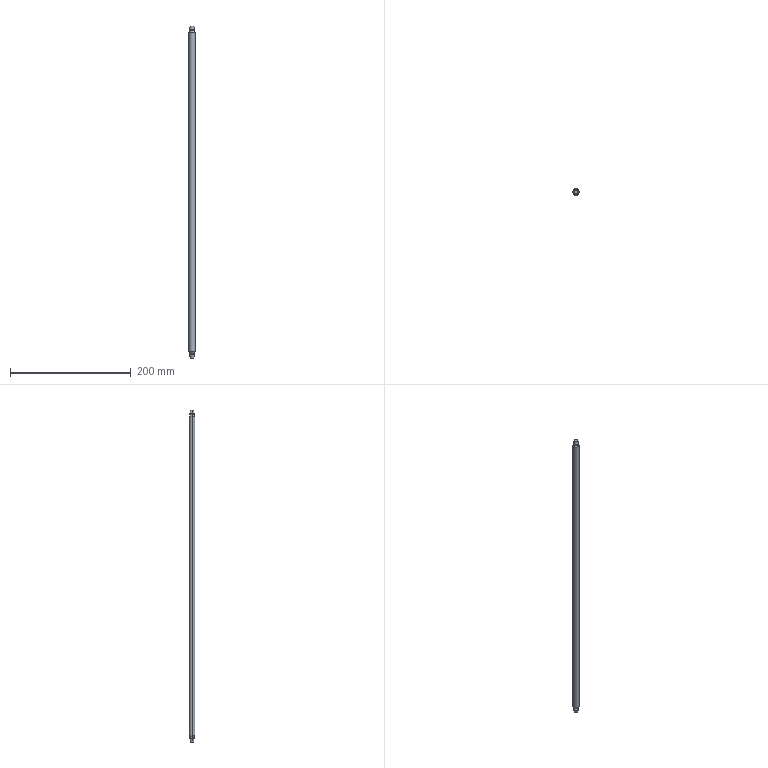Part | SolidWorks | features BaseBody 1 | 1 solid | 16 faces | box 10 x 10 x 550 mm | volume 42463 mm3 | torus 8 | cone 4 | cylinder 2 | plane 2 | commonest cylinder face diameters 10 x2
STEP:
#1=CARTESIAN_POINT('',(-5.,0.,-265.));
#2=VERTEX_POINT('',#1);
#3=CARTESIAN_POINT('',(-3.,0.,-267.));
#4=VERTEX_POINT('',#3);
#5=CARTESIAN_POINT('',(-5.,0.,-267.));
#6=DIRECTION('',(0.,1.,0.));
#7=DIRECTION('',(0.,0.,1.));
#8=AXIS2_PLACEMENT_3D('',#5,#6,#7);
#9=CIRCLE('',#8,2.);
#10=EDGE_CURVE('',#2,#4,#9,.T.);
#11=ORIENTED_EDGE('',*,*,#10,.T.);
#12=CARTESIAN_POINT('',(3.,0.,-267.));
#13=VERTEX_POINT('',#12);
#14=CARTESIAN_POINT('',(0.,0.,-267.));
#15=DIRECTION('',(0.,0.,1.));
#16=DIRECTION('',(1.,0.,0.));
#17=AXIS2_PLACEMENT_3D('',#14,#15,#16);
#18=CIRCLE('',#17,3.);
#19=EDGE_CURVE('',#4,#13,#18,.T.);
#20=ORIENTED_EDGE('',*,*,#19,.T.);
#21=CARTESIAN_POINT('',(5.,0.,-265.));
#22=VERTEX_POINT('',#21);
#23=CARTESIAN_POINT('',(5.,0.,-267.));
#24=DIRECTION('',(0.,-1.,0.));
#25=DIRECTION('',(1.,0.,0.));
#26=AXIS2_PLACEMENT_3D('',#23,#24,#25);
#27=CIRCLE('',#26,2.);
#28=EDGE_CURVE('',#22,#13,#27,.T.);
#29=ORIENTED_EDGE('',*,*,#28,.F.);
#30=CARTESIAN_POINT('',(0.,0.,-265.));
#31=DIRECTION('',(0.,0.,-1.));
#32=DIRECTION('',(-1.,0.,0.));
#33=AXIS2_PLACEMENT_3D('',#30,#31,#32);
#34=CIRCLE('',#33,5.);
#35=EDGE_CURVE('',#22,#2,#34,.T.);
#36=ORIENTED_EDGE('',*,*,#35,.T.);
#37=EDGE_LOOP('',(#11,#20,#29,#36));
#38=FACE_OUTER_BOUND('',#37,.T.);
#39=CARTESIAN_POINT('',(0.,0.,-267.));
#40=DIRECTION('',(0.,0.,1.));
#41=DIRECTION('',(-1.,0.,0.));
#42=AXIS2_PLACEMENT_3D('',#39,#40,#41);
#43=TOROIDAL_SURFACE('',#42,5.,2.);
#44=ADVANCED_FACE('',(#38),#43,.F.);
#45=CARTESIAN_POINT('',(-5.,0.,265.));
#46=VERTEX_POINT('',#45);
#47=CARTESIAN_POINT('',(-3.,0.,267.));
#48=VERTEX_POINT('',#47);
#49=CARTESIAN_POINT('',(-5.,0.,267.));
#50=DIRECTION('',(0.,-1.,0.));
#51=DIRECTION('',(0.,0.,-1.));
#52=AXIS2_PLACEMENT_3D('',#49,#50,#51);
#53=CIRCLE('',#52,2.);
#54=EDGE_CURVE('',#46,#48,#53,.T.);
#55=ORIENTED_EDGE('',*,*,#54,.T.);
#56=CARTESIAN_POINT('',(3.,0.,267.));
#57=VERTEX_POINT('',#56);
#58=CARTESIAN_POINT('',(0.,0.,267.));
#59=DIRECTION('',(0.,0.,-1.));
#60=DIRECTION('',(-1.,0.,0.));
#61=AXIS2_PLACEMENT_3D('',#58,#59,#60);
#62=CIRCLE('',#61,3.);
#63=EDGE_CURVE('',#48,#57,#62,.T.);
#64=ORIENTED_EDGE('',*,*,#63,.T.);
#65=CARTESIAN_POINT('',(5.,0.,265.));
#66=VERTEX_POINT('',#65);
#67=CARTESIAN_POINT('',(5.,0.,267.));
#68=DIRECTION('',(0.,1.,0.));
#69=DIRECTION('',(-1.,0.,0.));
#70=AXIS2_PLACEMENT_3D('',#67,#68,#69);
#71=CIRCLE('',#70,2.);
#72=EDGE_CURVE('',#66,#57,#71,.T.);
#73=ORIENTED_EDGE('',*,*,#72,.F.);
#74=CARTESIAN_POINT('',(0.,0.,265.));
#75=DIRECTION('',(0.,0.,1.));
#76=DIRECTION('',(-1.,0.,0.));
#77=AXIS2_PLACEMENT_3D('',#74,#75,#76);
#78=CIRCLE('',#77,5.);
#79=EDGE_CURVE('',#66,#46,#78,.T.);
#80=ORIENTED_EDGE('',*,*,#79,.T.);
#81=EDGE_LOOP('',(#55,#64,#73,#80));
#82=FACE_OUTER_BOUND('',#81,.T.);
#83=CARTESIAN_POINT('',(0.,0.,267.));
#84=DIRECTION('',(0.,0.,-1.));
#85=DIRECTION('',(-1.,0.,0.));
#86=AXIS2_PLACEMENT_3D('',#83,#84,#85);
#87=TOROIDAL_SURFACE('',#86,5.,2.);
#88=ADVANCED_FACE('',(#82),#87,.F.);
#89=ORIENTED_EDGE('',*,*,#72,.T.);
#90=CARTESIAN_POINT('',(0.,0.,267.));
#91=DIRECTION('',(0.,0.,-1.));
#92=DIRECTION('',(-1.,0.,0.));
#93=AXIS2_PLACEMENT_3D('',#90,#91,#92);
#94=CIRCLE('',#93,3.);
#95=EDGE_CURVE('',#57,#48,#94,.T.);
#96=ORIENTED_EDGE('',*,*,#95,.T.);
#97=ORIENTED_EDGE('',*,*,#54,.F.);
#98=CARTESIAN_POINT('',(0.,0.,265.));
#99=DIRECTION('',(0.,0.,1.));
#100=DIRECTION('',(-1.,0.,0.));
#101=AXIS2_PLACEMENT_3D('',#98,#99,#100);
#102=CIRCLE('',#101,5.);
#103=EDGE_CURVE('',#46,#66,#102,.T.);
#104=ORIENTED_EDGE('',*,*,#103,.T.);
#105=EDGE_LOOP('',(#89,#96,#97,#104));
#106=FACE_OUTER_BOUND('',#105,.T.);
#107=CARTESIAN_POINT('',(0.,0.,267.));
#108=DIRECTION('',(0.,0.,-1.));
#109=DIRECTION('',(-1.,0.,0.));
#110=AXIS2_PLACEMENT_3D('',#107,#108,#109);
#111=TOROIDAL_SURFACE('',#110,5.,2.);
#112=ADVANCED_FACE('',(#106),#111,.F.);
#113=ORIENTED_EDGE('',*,*,#28,.T.);
#114=CARTESIAN_POINT('',(0.,0.,-267.));
#115=DIRECTION('',(0.,0.,1.));
#116=DIRECTION('',(1.,0.,0.));
#117=AXIS2_PLACEMENT_3D('',#114,#115,#116);
#118=CIRCLE('',#117,3.);
#119=EDGE_CURVE('',#13,#4,#118,.T.);
#120=ORIENTED_EDGE('',*,*,#119,.T.);
#121=ORIENTED_EDGE('',*,*,#10,.F.);
#122=CARTESIAN_POINT('',(0.,0.,-265.));
#123=DIRECTION('',(0.,0.,-1.));
#124=DIRECTION('',(-1.,0.,0.));
#125=AXIS2_PLACEMENT_3D('',#122,#123,#124);
#126=CIRCLE('',#125,5.);
#127=EDGE_CURVE('',#2,#22,#126,.T.);
#128=ORIENTED_EDGE('',*,*,#127,.T.);
#129=EDGE_LOOP('',(#113,#120,#121,#128));
#130=FACE_OUTER_BOUND('',#129,.T.);
#131=CARTESIAN_POINT('',(0.,0.,-267.));
#132=DIRECTION('',(0.,0.,1.));
#133=DIRECTION('',(-1.,0.,0.));
#134=AXIS2_PLACEMENT_3D('',#131,#132,#133);
#135=TOROIDAL_SURFACE('',#134,5.,2.);
#136=ADVANCED_FACE('',(#130),#135,.F.);
#137=ORIENTED_EDGE('',*,*,#119,.F.);
#138=CARTESIAN_POINT('',(4.515,0.,-268.94));
#139=VERTEX_POINT('',#138);
#140=CARTESIAN_POINT('',(5.,0.,-267.));
#141=DIRECTION('',(0.,-1.,0.));
#142=DIRECTION('',(1.,0.,0.));
#143=AXIS2_PLACEMENT_3D('',#140,#141,#142);
#144=CIRCLE('',#143,2.);
#145=EDGE_CURVE('',#13,#139,#144,.T.);
#146=ORIENTED_EDGE('',*,*,#145,.T.);
#147=CARTESIAN_POINT('',(-4.515,0.,-268.94));
#148=VERTEX_POINT('',#147);
#149=CARTESIAN_POINT('',(0.,0.,-268.94));
#150=DIRECTION('',(0.,0.,-1.));
#151=DIRECTION('',(1.,0.,0.));
#152=AXIS2_PLACEMENT_3D('',#149,#150,#151);
#153=CIRCLE('',#152,4.515);
#154=EDGE_CURVE('',#148,#139,#153,.T.);
#155=ORIENTED_EDGE('',*,*,#154,.F.);
#156=CARTESIAN_POINT('',(-5.,0.,-267.));
#157=DIRECTION('',(0.,1.,0.));
#158=DIRECTION('',(0.,0.,1.));
#159=AXIS2_PLACEMENT_3D('',#156,#157,#158);
#160=CIRCLE('',#159,2.);
#161=EDGE_CURVE('',#4,#148,#160,.T.);
#162=ORIENTED_EDGE('',*,*,#161,.F.);
#163=EDGE_LOOP('',(#137,#146,#155,#162));
#164=FACE_OUTER_BOUND('',#163,.T.);
#165=CARTESIAN_POINT('',(0.,0.,-267.));
#166=DIRECTION('',(0.,0.,1.));
#167=DIRECTION('',(-1.,0.,0.));
#168=AXIS2_PLACEMENT_3D('',#165,#166,#167);
#169=TOROIDAL_SURFACE('',#168,5.,2.);
#170=ADVANCED_FACE('',(#164),#169,.F.);
#171=ORIENTED_EDGE('',*,*,#95,.F.);
#172=CARTESIAN_POINT('',(4.515,0.,268.94));
#173=VERTEX_POINT('',#172);
#174=CARTESIAN_POINT('',(5.,0.,267.));
#175=DIRECTION('',(0.,1.,0.));
#176=DIRECTION('',(-1.,0.,0.));
#177=AXIS2_PLACEMENT_3D('',#174,#175,#176);
#178=CIRCLE('',#177,2.);
#179=EDGE_CURVE('',#57,#173,#178,.T.);
#180=ORIENTED_EDGE('',*,*,#179,.T.);
#181=CARTESIAN_POINT('',(-4.515,0.,268.94));
#182=VERTEX_POINT('',#181);
#183=CARTESIAN_POINT('',(0.,0.,268.94));
#184=DIRECTION('',(0.,0.,-1.));
#185=DIRECTION('',(1.,0.,0.));
#186=AXIS2_PLACEMENT_3D('',#183,#184,#185);
#187=CIRCLE('',#186,4.515);
#188=EDGE_CURVE('',#173,#182,#187,.T.);
#189=ORIENTED_EDGE('',*,*,#188,.T.);
#190=CARTESIAN_POINT('',(-5.,0.,267.));
#191=DIRECTION('',(0.,-1.,0.));
#192=DIRECTION('',(0.,0.,-1.));
#193=AXIS2_PLACEMENT_3D('',#190,#191,#192);
#194=CIRCLE('',#193,2.);
#195=EDGE_CURVE('',#48,#182,#194,.T.);
#196=ORIENTED_EDGE('',*,*,#195,.F.);
#197=EDGE_LOOP('',(#171,#180,#189,#196));
#198=FACE_OUTER_BOUND('',#197,.T.);
#199=CARTESIAN_POINT('',(0.,0.,267.));
#200=DIRECTION('',(0.,0.,-1.));
#201=DIRECTION('',(-1.,0.,0.));
#202=AXIS2_PLACEMENT_3D('',#199,#200,#201);
#203=TOROIDAL_SURFACE('',#202,5.,2.);
#204=ADVANCED_FACE('',(#198),#203,.F.);
#205=CARTESIAN_POINT('',(3.,0.,-275.));
#206=VERTEX_POINT('',#205);
#207=CARTESIAN_POINT('',(-3.,0.,-275.));
#208=VERTEX_POINT('',#207);
#209=CARTESIAN_POINT('',(0.,0.,-275.));
#210=DIRECTION('',(0.,0.,-1.));
#211=DIRECTION('',(1.,0.,0.));
#212=AXIS2_PLACEMENT_3D('',#209,#210,#211);
#213=CIRCLE('',#212,3.);
#214=EDGE_CURVE('',#206,#208,#213,.T.);
#215=ORIENTED_EDGE('',*,*,#214,.F.);
#216=CARTESIAN_POINT('',(3.757,0.,-271.97));
#217=DIRECTION('',(0.2425,0.,0.9701));
#218=VECTOR('',#217,1000.);
#219=LINE('',#216,#218);
#220=EDGE_CURVE('',#206,#139,#219,.T.);
#221=ORIENTED_EDGE('',*,*,#220,.T.);
#222=CARTESIAN_POINT('',(0.,0.,-268.94));
#223=DIRECTION('',(0.,0.,-1.));
#224=DIRECTION('',(1.,0.,0.));
#225=AXIS2_PLACEMENT_3D('',#222,#223,#224);
#226=CIRCLE('',#225,4.515);
#227=EDGE_CURVE('',#139,#148,#226,.T.);
#228=ORIENTED_EDGE('',*,*,#227,.T.);
#229=CARTESIAN_POINT('',(-3.757,0.,-271.97));
#230=DIRECTION('',(-0.2425,0.,0.9701));
#231=VECTOR('',#230,1000.);
#232=LINE('',#229,#231);
#233=EDGE_CURVE('',#208,#148,#232,.T.);
#234=ORIENTED_EDGE('',*,*,#233,.F.);
#235=EDGE_LOOP('',(#215,#221,#228,#234));
#236=FACE_OUTER_BOUND('',#235,.T.);
#237=CARTESIAN_POINT('',(0.,0.,-271.97));
#238=DIRECTION('',(0.,0.,1.));
#239=DIRECTION('',(-1.,0.,0.));
#240=AXIS2_PLACEMENT_3D('',#237,#238,#239);
#241=CONICAL_SURFACE('',#240,3.757,0.245);
#242=ADVANCED_FACE('',(#236),#241,.T.);
#243=CARTESIAN_POINT('',(-3.,0.,275.));
#244=VERTEX_POINT('',#243);
#245=CARTESIAN_POINT('',(3.,0.,275.));
#246=VERTEX_POINT('',#245);
#247=CARTESIAN_POINT('',(0.,0.,275.));
#248=DIRECTION('',(0.,0.,-1.));
#249=DIRECTION('',(1.,0.,0.));
#250=AXIS2_PLACEMENT_3D('',#247,#248,#249);
#251=CIRCLE('',#250,3.);
#252=EDGE_CURVE('',#244,#246,#251,.T.);
#253=ORIENTED_EDGE('',*,*,#252,.T.);
#254=CARTESIAN_POINT('',(3.757,0.,271.97));
#255=DIRECTION('',(0.2425,0.,-0.9701));
#256=VECTOR('',#255,1000.);
#257=LINE('',#254,#256);
#258=EDGE_CURVE('',#246,#173,#257,.T.);
#259=ORIENTED_EDGE('',*,*,#258,.T.);
#260=CARTESIAN_POINT('',(0.,0.,268.94));
#261=DIRECTION('',(0.,0.,-1.));
#262=DIRECTION('',(1.,0.,0.));
#263=AXIS2_PLACEMENT_3D('',#260,#261,#262);
#264=CIRCLE('',#263,4.515);
#265=EDGE_CURVE('',#182,#173,#264,.T.);
#266=ORIENTED_EDGE('',*,*,#265,.F.);
#267=CARTESIAN_POINT('',(-3.757,0.,271.97));
#268=DIRECTION('',(-0.2425,0.,-0.9701));
#269=VECTOR('',#268,1000.);
#270=LINE('',#267,#269);
#271=EDGE_CURVE('',#244,#182,#270,.T.);
#272=ORIENTED_EDGE('',*,*,#271,.F.);
#273=EDGE_LOOP('',(#253,#259,#266,#272));
#274=FACE_OUTER_BOUND('',#273,.T.);
#275=CARTESIAN_POINT('',(0.,0.,271.97));
#276=DIRECTION('',(0.,0.,-1.));
#277=DIRECTION('',(-1.,0.,0.));
#278=AXIS2_PLACEMENT_3D('',#275,#276,#277);
#279=CONICAL_SURFACE('',#278,3.757,0.245);
#280=ADVANCED_FACE('',(#274),#279,.T.);
#281=ORIENTED_EDGE('',*,*,#79,.F.);
#282=CARTESIAN_POINT('',(5.,0.,0.));
#283=DIRECTION('',(0.,0.,-1.));
#284=VECTOR('',#283,1000.);
#285=LINE('',#282,#284);
#286=EDGE_CURVE('',#66,#22,#285,.T.);
#287=ORIENTED_EDGE('',*,*,#286,.T.);
#288=ORIENTED_EDGE('',*,*,#127,.F.);
#289=CARTESIAN_POINT('',(-5.,0.,0.));
#290=DIRECTION('',(0.,0.,-1.));
#291=VECTOR('',#290,1000.);
#292=LINE('',#289,#291);
#293=EDGE_CURVE('',#46,#2,#292,.T.);
#294=ORIENTED_EDGE('',*,*,#293,.F.);
#295=EDGE_LOOP('',(#281,#287,#288,#294));
#296=FACE_OUTER_BOUND('',#295,.T.);
#297=CARTESIAN_POINT('',(0.,0.,0.));
#298=DIRECTION('',(0.,0.,-1.));
#299=DIRECTION('',(-1.,0.,0.));
#300=AXIS2_PLACEMENT_3D('',#297,#298,#299);
#301=CYLINDRICAL_SURFACE('',#300,5.);
#302=ADVANCED_FACE('',(#296),#301,.T.);
#303=CARTESIAN_POINT('',(0.,0.,-275.));
#304=DIRECTION('',(0.,0.,-1.));
#305=DIRECTION('',(1.,0.,0.));
#306=AXIS2_PLACEMENT_3D('',#303,#304,#305);
#307=CIRCLE('',#306,3.);
#308=EDGE_CURVE('',#208,#206,#307,.T.);
#309=ORIENTED_EDGE('',*,*,#308,.T.);
#310=ORIENTED_EDGE('',*,*,#214,.T.);
#311=EDGE_LOOP('',(#309,#310));
#312=FACE_OUTER_BOUND('',#311,.T.);
#313=CARTESIAN_POINT('',(-3.,0.,-275.));
#314=DIRECTION('',(0.,0.,1.));
#315=DIRECTION('',(1.,0.,0.));
#316=AXIS2_PLACEMENT_3D('',#313,#314,#315);
#317=PLANE('',#316);
#318=ADVANCED_FACE('',(#312),#317,.F.);
#319=ORIENTED_EDGE('',*,*,#252,.F.);
#320=CARTESIAN_POINT('',(0.,0.,275.));
#321=DIRECTION('',(0.,0.,-1.));
#322=DIRECTION('',(1.,0.,0.));
#323=AXIS2_PLACEMENT_3D('',#320,#321,#322);
#324=CIRCLE('',#323,3.);
#325=EDGE_CURVE('',#246,#244,#324,.T.);
#326=ORIENTED_EDGE('',*,*,#325,.F.);
#327=EDGE_LOOP('',(#319,#326));
#328=FACE_OUTER_BOUND('',#327,.T.);
#329=CARTESIAN_POINT('',(-3.,0.,275.));
#330=DIRECTION('',(0.,0.,1.));
#331=DIRECTION('',(1.,0.,0.));
#332=AXIS2_PLACEMENT_3D('',#329,#330,#331);
#333=PLANE('',#332);
#334=ADVANCED_FACE('',(#328),#333,.T.);
#335=ORIENTED_EDGE('',*,*,#286,.F.);
#336=ORIENTED_EDGE('',*,*,#103,.F.);
#337=ORIENTED_EDGE('',*,*,#293,.T.);
#338=ORIENTED_EDGE('',*,*,#35,.F.);
#339=EDGE_LOOP('',(#335,#336,#337,#338));
#340=FACE_OUTER_BOUND('',#339,.T.);
#341=CARTESIAN_POINT('',(0.,0.,0.));
#342=DIRECTION('',(0.,0.,-1.));
#343=DIRECTION('',(-1.,0.,0.));
#344=AXIS2_PLACEMENT_3D('',#341,#342,#343);
#345=CYLINDRICAL_SURFACE('',#344,5.);
#346=ADVANCED_FACE('',(#340),#345,.T.);
#347=ORIENTED_EDGE('',*,*,#258,.F.);
#348=ORIENTED_EDGE('',*,*,#325,.T.);
#349=ORIENTED_EDGE('',*,*,#271,.T.);
#350=ORIENTED_EDGE('',*,*,#188,.F.);
#351=EDGE_LOOP('',(#347,#348,#349,#350));
#352=FACE_OUTER_BOUND('',#351,.T.);
#353=CARTESIAN_POINT('',(0.,0.,271.97));
#354=DIRECTION('',(0.,0.,-1.));
#355=DIRECTION('',(-1.,0.,0.));
#356=AXIS2_PLACEMENT_3D('',#353,#354,#355);
#357=CONICAL_SURFACE('',#356,3.757,0.245);
#358=ADVANCED_FACE('',(#352),#357,.T.);
#359=ORIENTED_EDGE('',*,*,#220,.F.);
#360=ORIENTED_EDGE('',*,*,#308,.F.);
#361=ORIENTED_EDGE('',*,*,#233,.T.);
#362=ORIENTED_EDGE('',*,*,#154,.T.);
#363=EDGE_LOOP('',(#359,#360,#361,#362));
#364=FACE_OUTER_BOUND('',#363,.T.);
#365=CARTESIAN_POINT('',(0.,0.,-271.97));
#366=DIRECTION('',(0.,0.,1.));
#367=DIRECTION('',(-1.,0.,0.));
#368=AXIS2_PLACEMENT_3D('',#365,#366,#367);
#369=CONICAL_SURFACE('',#368,3.757,0.245);
#370=ADVANCED_FACE('',(#364),#369,.T.);
#371=ORIENTED_EDGE('',*,*,#63,.F.);
#372=ORIENTED_EDGE('',*,*,#195,.T.);
#373=ORIENTED_EDGE('',*,*,#265,.T.);
#374=ORIENTED_EDGE('',*,*,#179,.F.);
#375=EDGE_LOOP('',(#371,#372,#373,#374));
#376=FACE_OUTER_BOUND('',#375,.T.);
#377=CARTESIAN_POINT('',(0.,0.,267.));
#378=DIRECTION('',(0.,0.,-1.));
#379=DIRECTION('',(-1.,0.,0.));
#380=AXIS2_PLACEMENT_3D('',#377,#378,#379);
#381=TOROIDAL_SURFACE('',#380,5.,2.);
#382=ADVANCED_FACE('',(#376),#381,.F.);
#383=ORIENTED_EDGE('',*,*,#19,.F.);
#384=ORIENTED_EDGE('',*,*,#161,.T.);
#385=ORIENTED_EDGE('',*,*,#227,.F.);
#386=ORIENTED_EDGE('',*,*,#145,.F.);
#387=EDGE_LOOP('',(#383,#384,#385,#386));
#388=FACE_OUTER_BOUND('',#387,.T.);
#389=CARTESIAN_POINT('',(0.,0.,-267.));
#390=DIRECTION('',(0.,0.,1.));
#391=DIRECTION('',(-1.,0.,0.));
#392=AXIS2_PLACEMENT_3D('',#389,#390,#391);
#393=TOROIDAL_SURFACE('',#392,5.,2.);
#394=ADVANCED_FACE('',(#388),#393,.F.);
#395=CLOSED_SHELL('',(#44,#88,#112,#136,#170,#204,#242,#280,#302,#318,#334,#346,#358,#370,#382,#394));
#396=MANIFOLD_SOLID_BREP('',#395);
#397=CARTESIAN_POINT('',(0.,0.,0.));
#398=DIRECTION('',(0.,0.,1.));
#399=DIRECTION('',(1.,0.,0.));
#400=AXIS2_PLACEMENT_3D('',#397,#398,#399);
#401=(LENGTH_UNIT()NAMED_UNIT(*)SI_UNIT(.MILLI.,.METRE.));
#402=UNCERTAINTY_MEASURE_WITH_UNIT(LENGTH_MEASURE(0.00001),#401,'','');
#403=(NAMED_UNIT(*)PLANE_ANGLE_UNIT()SI_UNIT($,.RADIAN.));
#404=(NAMED_UNIT(*)SI_UNIT($,.STERADIAN.)SOLID_ANGLE_UNIT());
#405=(GEOMETRIC_REPRESENTATION_CONTEXT(3)GLOBAL_UNCERTAINTY_ASSIGNED_CONTEXT((#402))GLOBAL_UNIT_ASSIGNED_CONTEXT((#401,#403,#404))REPRESENTATION_CONTEXT('',''));
#406=ADVANCED_BREP_SHAPE_REPRESENTATION('',(#396,#400),#405);